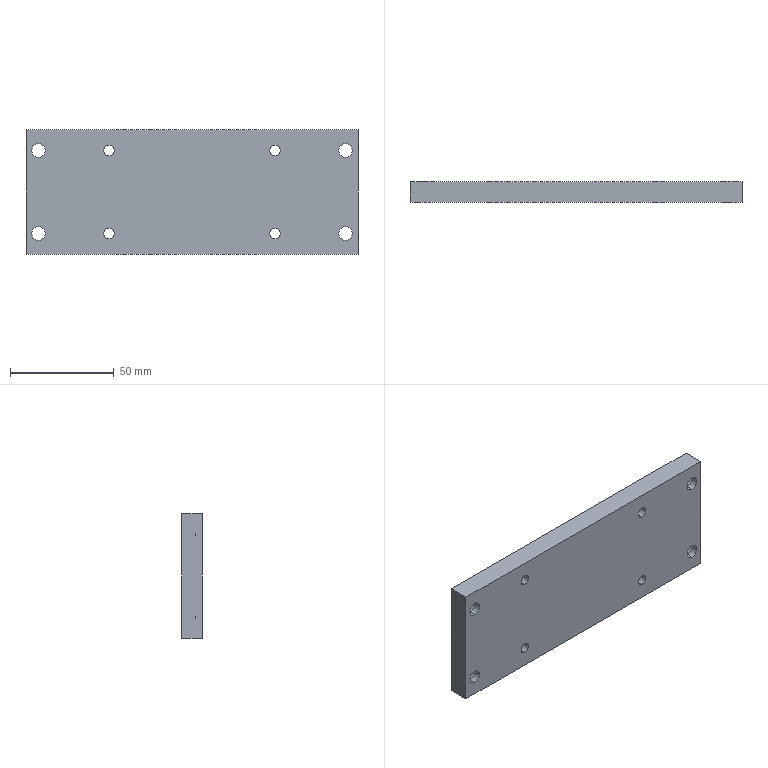Part | STEP file | Tube support mounting bracket top plate | 1 solid | 34 faces | box 160 x 10 x 60 mm | volume 92192 mm3 | cylinder 24 | plane 10 | commonest cylinder face diameters 5 x8 6.6 x8 11 x8